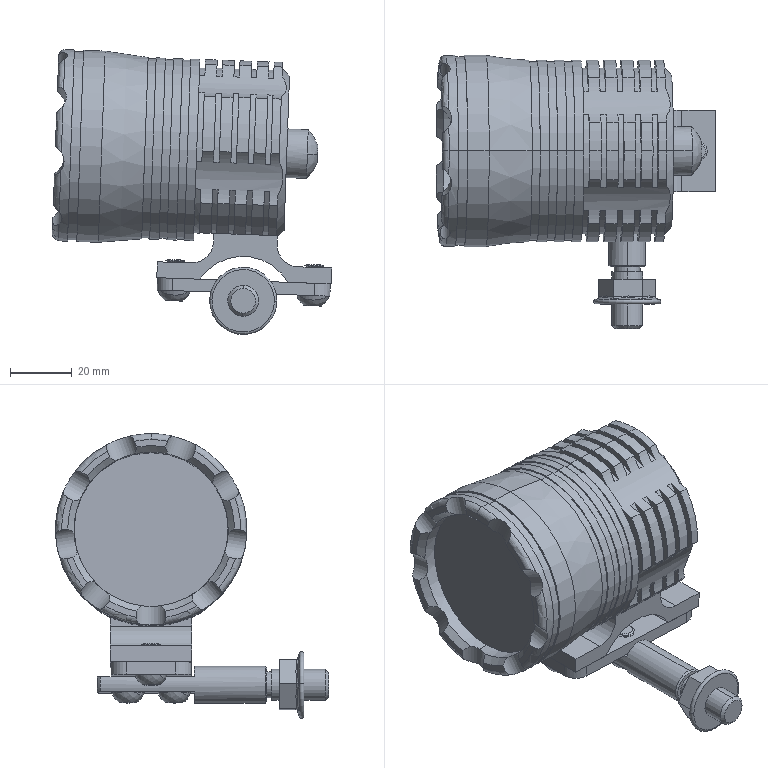Part | SolidWorks | features BaseBody 1 | 1 solid | 520 faces | box 90.524 x 88.5 x 92.29 mm | volume 184653 mm3 | plane 178 | cylinder 165 | cone 125 | sphere 22 | spline 18 | torus 12 | commonest cylinder face diameters 6 x48 58.8 x36 53.718 x25 10.407 x9 6.5 x8 10 x8